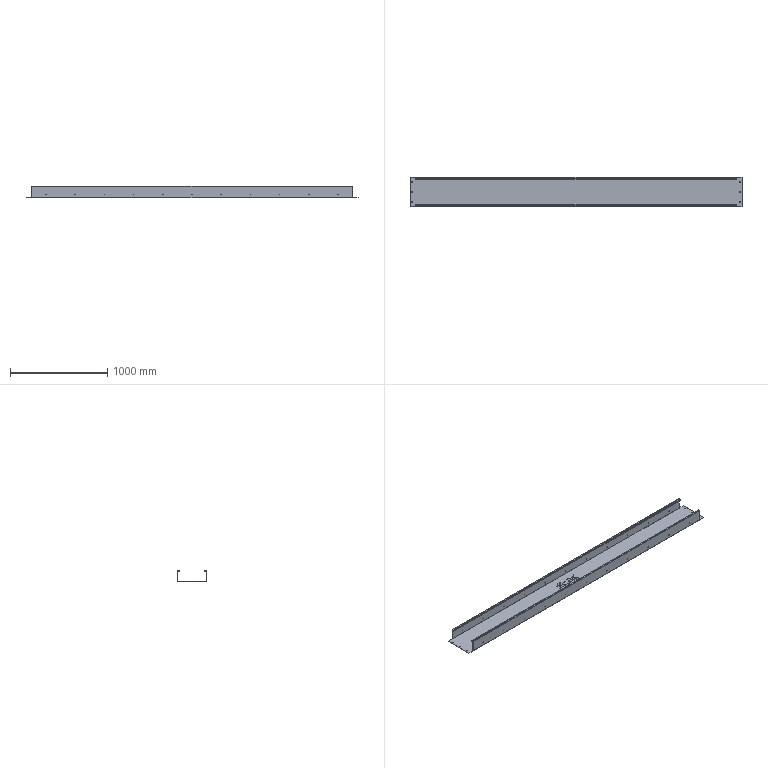Part | STEP file | TS-S95 TBD | 1 solid | 278 faces | box 3411 x 300 x 120 mm | volume 3926160 mm3 | plane 133 | cylinder 112 | spline 33 | commonest cylinder face diameters 5.4 x88 7 x12 0.4 x6 4.4 x6